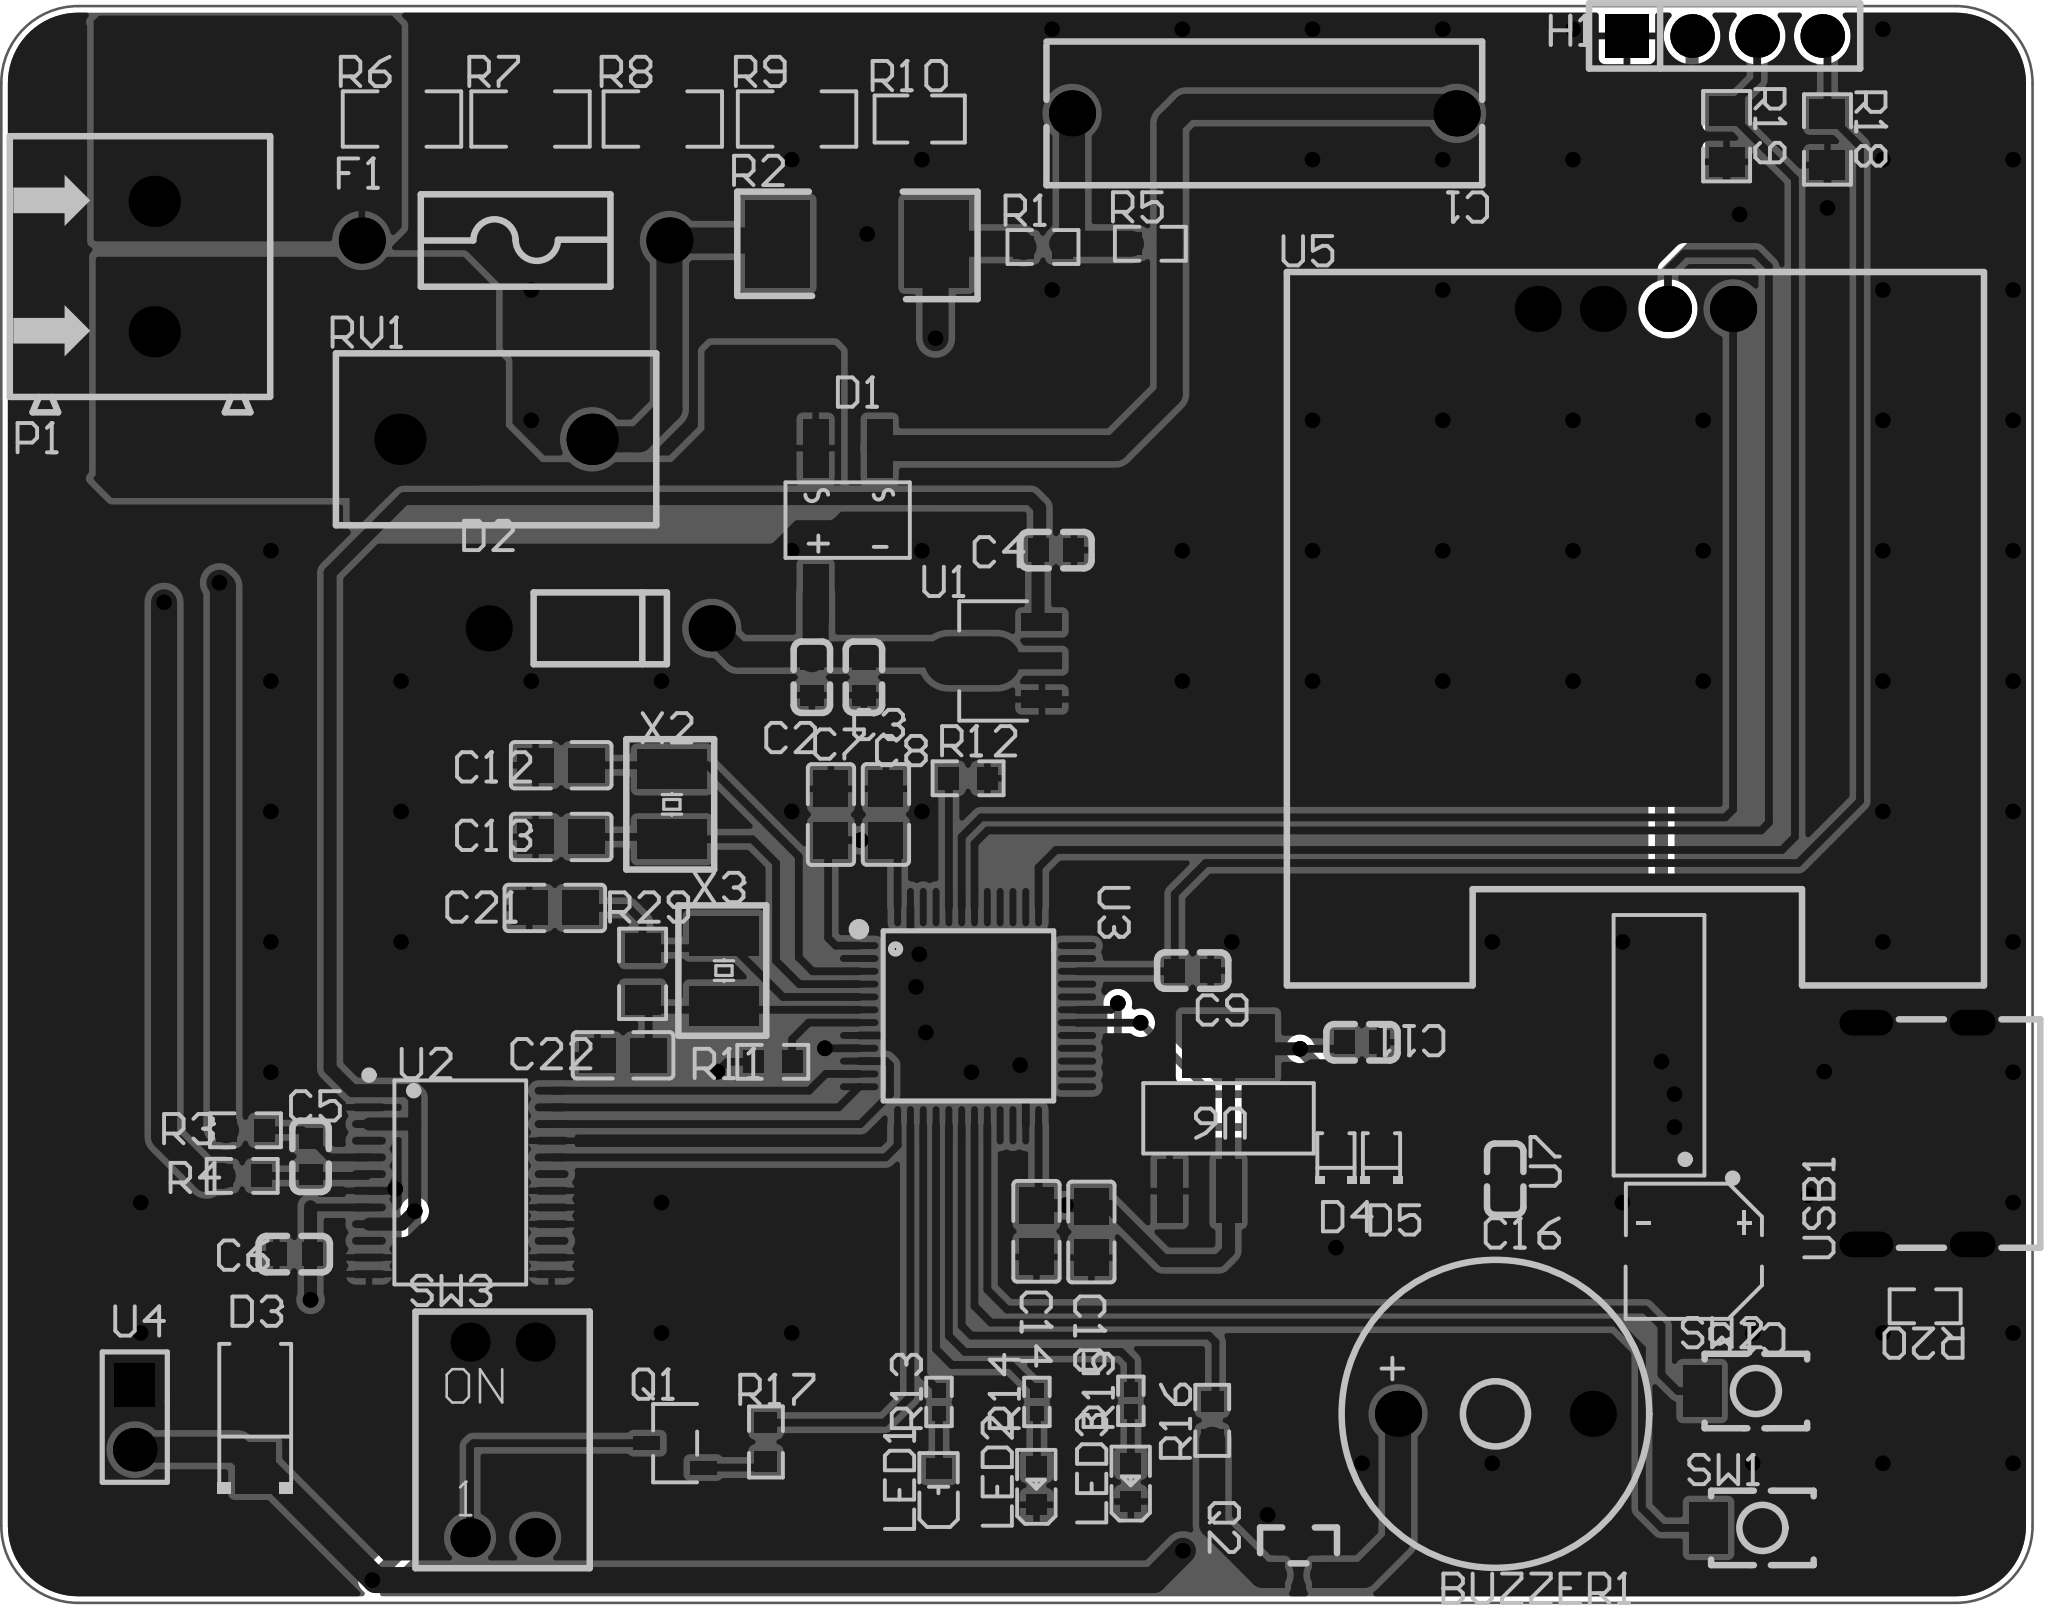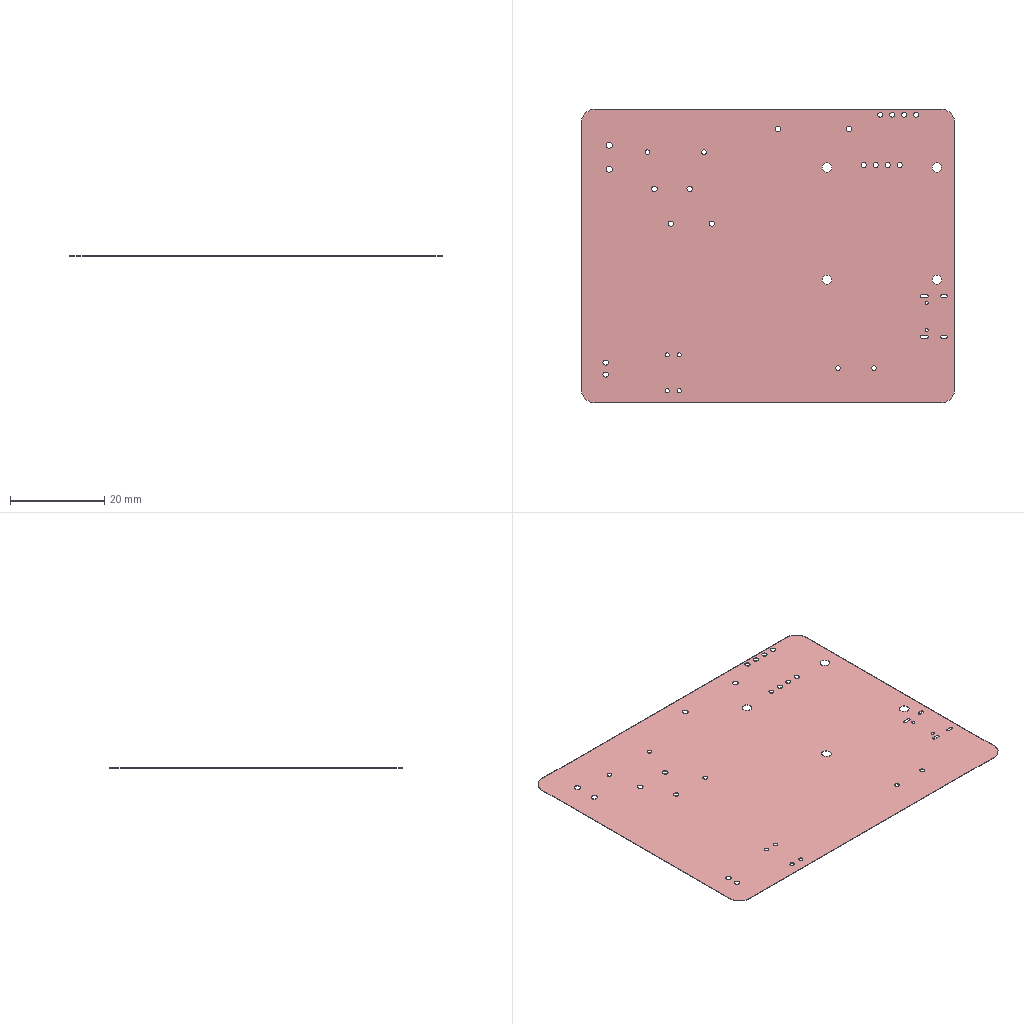Circuit board layout | Altium Designer | box 79.2 x 62.2 x 0.1 mm
Layer stack:
# Altium Designer layer stack of  (unit mm; dielectric type: 0 none, 1 core, 2 prepreg, 3 surface material)
index,name,kind,layer,copper_thickness_mm,dielectric_type,dielectric_thickness_mm,dielectric_material,dielectric_constant
0,Top Paste Mask Layer,other,,,,,,
1,Top Silkscreen Layer,other,,,,,,
2,Top Solder Mask Layer,dielectric,,,3,0.01,,3.3
3,Top Layer,copper,Top Layer,0.035,,,,
4,Bottom Layer,copper,Bottom Layer,0.035,,,,
5,Bottom Solder Mask Layer,dielectric,,,3,0.01,,3.3
6,Bottom Silkscreen Layer,other,,,,,,
7,Bottom Paste Mask Layer,other,,,,,,
# drill layer pairs: low layer,high layer
drill_pair,Top Layer,Bottom Layer
Part placement:
Designator,Comment,Layer,Footprint,Center-X(mm),Center-Y(mm),Rotation
BUZZER1,2.4kHz,TopLayer,BUZ-TH_BD12.0-P7.60-D0.6-FD,140.589,89.281,0
C1,470nF,TopLayer,CAP-TH_L17.0-W5.5-P15.00-D1.2,131.572,139.954,180
C2,100µF,TopLayer,C0603,113.919,117.983,90
C3,0.1µF,TopLayer,C0603,115.951,117.983,270
C4,10µF,TopLayer,C0603,123.444,122.936,180
C5,1nF,TopLayer,C0603,94.361,99.314,90
C6,1nF,TopLayer,C0603,93.726,95.504,0
C7,100nF,TopLayer,C0805,114.665,112.633,90
C8,100nF,TopLayer,C0805,116.809,112.637,270
C14,100nF,TopLayer,C0805,122.682,96.393,90
C10,100nF,TopLayer,C0805,124.825,96.367,270
C11,100nF,TopLayer,C0603,135.382,103.759,180
D1,MB10S,TopLayer,MBS_L4.7-W4.0-P2.50-LS7.0-TL,115.316,124.079,270
D2,1N4742,TopLayer,DO-41_BD2.4-L4.7-P8.70-D0.8-FD,105.664,119.888,0
D3,1N4007,TopLayer,SMA_L4.3-W2.5-LS5.0-RD,92.202,89.281,90
F1,2F0.05002S1B02,TopLayer,FUSE-TH_BD3.0-L7.2-P11.20-D0.6,102.362,135.001,0
LED1,NCD0603G1,TopLayer,LED0603-RD_1,118.869,86.361,90
LED2,NCD0603R1,TopLayer,LED0603-RD_RED,122.682,86.487,90
LED3,NCD0603Y1,TopLayer,LED0603-RD,126.365,86.614,90
Q1,S8050 J3Y(RANGE:200-350),TopLayer,SOT-23-3_L3.0-W1.7-P0.95-LS2.9-BR,108.585,88.138,0
R1,10Ω,TopLayer,R0603,122.936,134.747,0
R2,2mΩ,TopLayer,RES-SMD_L6.4-W3.2-1,115.697,134.874,0
R3,1K,TopLayer,R0603,91.821,100.33,0
R4,1K,TopLayer,R0603,91.694,98.552,0
R5,1MΩ,TopLayer,R0603,127.127,134.874,0
R6,1MΩ,TopLayer,R1206,97.928,139.734,0
R7,1MΩ,TopLayer,R1206,102.943,139.734,0
R8,1MΩ,TopLayer,R1206,108.104,139.734,0
R9,1MΩ,TopLayer,R1206,113.342,139.734,0
R10,10kΩ,TopLayer,R0805,118.127,139.734,0
R11,10K,TopLayer,R0603,112.395,102.997,0
R12,10K,TopLayer,R0603,120.015,114.046,0
R13,220Ω,TopLayer,R0402,118.879,89.745,90
R14,220Ω,TopLayer,R0402,122.7,89.745,90
R15,220Ω,TopLayer,R0402,126.365,89.789,90
R16,1KΩ,TopLayer,R0603,129.54,89.027,90
R17,1KΩ,TopLayer,R0603,112.128,88.184,270
RV1,190pF@1kHz,TopLayer,RES-TH_L12.5-W6.7-P7.50-D1.2,101.6,127.254,0
SW1,TS3425A2P 250gf,TopLayer,SW-SMD_L3.9-W2.9-LS5.0,151.003,84.836,0
SW2,TS3425A2P 250gf,TopLayer,SW-SMD_L3.9-W2.9-LS5.0,150.749,90.17,0
SW3,BSE02GR,TopLayer,SW-TH_4P-L9.9-W6.8-P7.62-BL,101.854,88.265,0
U1,HT7550-1,TopLayer,SOT-89_L4.5-W2.5-P1.50-LS4.2-BR,121.734,118.618,0
U2,ADE7755ARSZ,TopLayer,SSOP-24_L8.1-W5.3-P0.65-LS7.8-BL,100.203,98.298,270
U3,STM32F030C8T6TR,TopLayer,LQFP-48_L7.0-W7.0-P0.50-LS9.0-BL,120.015,104.775,270
U5,HS96L03W2C03,TopLayer,OLED-TH_L27.8-W27.2-P2.54_C9900033791,146.05,132.334,0
U6,AMS1117-3.3,TopLayer,SOT-223-4_L6.5-W3.5-P2.30-LS7.0-BR,130.175,100.796,270
P1,WJ500V-5.08-2P,TopLayer,CONN-TH_2P-P5.00_WJ500V-5.08-2P,88.265,133.985,90
U4,KF301-5.0-2P,TopLayer,HDR-M-2.54_1X2,87.503,89.154,270
C12,20pF,TopLayer,C0805,104.14,114.554,180
C13,20pF,TopLayer,C0805,104.14,111.76,0
C21,20pF,TopLayer,C0805,103.891,108.994,0
C22,20pF,TopLayer,C0805,106.553,103.251,0
R29,1M,TopLayer,R0805,107.315,106.426,90
X2,32.768MHz,TopLayer,CRYSTAL-SMD_L3.2-W2.5_3225-8MHZ,108.458,113.03,90
X3,8MHz,TopLayer,CRYSTAL-SMD_L3.2-W2.5_3225-8MHZ,110.49,106.553,90
C9,100nF,TopLayer,C0603,128.778,106.553,180
C15,10uF,TopLayer,CAP-SMD_BD5.0-L5.3-W5.3-FD,148.327,95.631,180
C16,100nF,TopLayer,C0603,140.97,98.425,90
R18,10kΩ,TopLayer,R0805,153.543,138.938,270
R19,10kΩ,TopLayer,R0805,149.606,139.065,270
R20,5.1K,TopLayer,R0603,157.353,93.472,180
U7,CH340C,TopLayer,SOP-16_L10.0-W3.9-P1.27-LS6.0-BL,146.97,103.642,90
USB1,TYPE-C16PIN,TopLayer,USB-C-SMD_TYPE-C16PIN,156.845,100.203,90
Q2,,TopLayer,S8050_SOT-23,132.906,84.154,270
H1,,TopLayer,HDR-TH_4P-P2.54-V-F,149.53,142.971,0
D4,1N5819WS,TopLayer,SOD-323_L1.8-W1.3-LS2.5-RD,134.366,99.314,90
D5,1N5819WS,TopLayer,SOD-323_L1.8-W1.3-LS2.5-RD,136.144,99.314,90
Pad and via stacks:
# Altium Designer via and pad stacks of  (unit mm). Each distinct definition once, with the count of objects using it.
# via: kind,start_layer,end_layer,hole_mm,diameter_mm,mode(0 simple;1 top-mid-bottom;2 full stack),diameter_per_layer,count,example_net
# pad: kind,layer,hole_mm,hole_type(0 round;1 square;2 slot),plating,top_size,top_shape(1 round;2 rect;3 octagon;9 rounded rect),mid_size,bottom_size,mode,footprint,size_per_layer,count,example
pad,Multi-Layer,1,0,plated,1.8x1.8,1,1.8x1.8,1.8x1.8,0,BUZ-TH_BD12.0-P7.60-D0.6-FD,,2,BUZZER1.2
pad,Multi-Layer,1.2,0,plated,1.8x1.8,1,1.8x1.8,1.8x1.8,0,CAP-TH_L17.0-W5.5-P15.00-D1.2,,2,C1.1
pad,Multi-Layer,1.1,0,plated,1.8x1.8,1,1.8x1.8,1.8x1.8,0,DO-41_BD2.4-L4.7-P8.70-D0.8-FD,,2,D2.1
pad,Multi-Layer,1,0,plated,1.8x1.8,1,1.8x1.8,1.8x1.8,0,FUSE-TH_BD3.0-L7.2-P11.20-D0.6,,2,F1.1
pad,Multi-Layer,1.2,0,plated,2x2,1,2x2,2x2,0,RES-TH_L12.5-W6.7-P7.50-D1.2,,2,RV1.1
pad,Multi-Layer,0.9144,0,plated,1.524x1.524,1,1.524x1.524,1.524x1.524,0,SW-TH_4P-L9.9-W6.8-P7.62-BL,,4,SW3.1
pad,Multi-Layer,1.05,0,plated,1.8x1.8,1,1.8x1.8,1.8x1.8,0,OLED-TH_L27.8-W27.2-P2.54_C9900033791,,4,U5.1
pad,Multi-Layer,1.3,0,plated,2x2,1,2x2,2x2,0,CONN-TH_2P-P5.00_WJ500V-5.08-2P,,2,P1.2
pad,Multi-Layer,1.1,0,plated,1.7x1.575,2,1.7x1.575,1.7x1.575,0,HDR-M-2.54_1X2,,1,U4.1
pad,Multi-Layer,1.1,0,plated,1.7x1.7,1,1.7x1.7,1.7x1.7,0,HDR-M-2.54_1X2,,1,U4.2
pad,Multi-Layer,0.6,2,plated,1x1.8,1,1x1.8,1x1.8,0,USB-C-SMD_TYPE-C16PIN,,2,USB1.4
pad,Multi-Layer,0.6,2,plated,1x2.1,1,1x2.1,1x2.1,0,USB-C-SMD_TYPE-C16PIN,,2,USB1.2
pad,Multi-Layer,1.1,0,plated,1.7x1.7,2,1.7x1.7,1.7x1.7,0,HDR-TH_4P-P2.54-V-F,,1,H1.1
pad,Multi-Layer,1.1,0,plated,1.7x1.7,1,1.7x1.7,1.7x1.7,0,HDR-TH_4P-P2.54-V-F,,3,H1.2
pad,Top Layer,0,0,plated,0.8x0.9,2,0.8x0.9,0.8x0.9,0,C0603,,16,C2.2
pad,Top Layer,0,0,plated,1.41x1.35,2,1.41x1.35,1.41x1.35,0,C0805,,16,C7.2
pad,Top Layer,0,0,plated,0.98x2.265,2,0.98x2.265,0.98x2.265,0,MBS_L4.7-W4.0-P2.50-LS7.0-TL,,4,D1.1
pad,Top Layer,0,0,plated,2x1.593,2,2x1.593,2x1.593,0,SMA_L4.3-W2.5-LS5.0-RD,,2,D3.2
pad,Top Layer,0,0,plated,1x0.8,2,1x0.8,1x0.8,0,LED0603-RD_1,,2,LED1.2
pad,Top Layer,0,0,plated,0.8x0.8,2,0.8x0.8,0.8x0.8,0,LED0603-RD_RED,,2,LED2.1
pad,Top Layer,0,0,plated,0.8x0.8,2,0.8x0.8,0.8x0.8,0,LED0603-RD,,2,LED3.2
pad,Top Layer,0,0,plated,1.038x0.532,2,1.038x0.532,1.038x0.532,0,SOT-23-3_L3.0-W1.7-P0.95-LS2.9-BR,,3,Q1.1
pad,Top Layer,0,0,plated,0.8065x0.864,2,0.8065x0.864,0.8065x0.864,0,R0603,,18,R1.2
pad,Top Layer,0,0,plated,2.5x3.4,2,2.5x3.4,2.5x3.4,0,RES-SMD_L6.4-W3.2-1,,2,R2.2
pad,Top Layer,0,0,plated,1.208x1.701,2,1.208x1.701,1.208x1.701,0,R1206,,8,R6.2
pad,Top Layer,0,0,plated,1.133x1.377,2,1.133x1.377,1.133x1.377,0,R0805,,8,R10.2
pad,Top Layer,0,0,plated,0.5657x0.54,2,0.5657x0.54,0.5657x0.54,0,R0402,,6,R13.2
pad,Top Layer,0,0,plated,1.5x2,2,1.5x2,1.5x2,0,SW-SMD_L3.9-W2.9-LS5.0,,4,SW1.1
pad,Top Layer,0,0,plated,0.95x0.95,1,0.95x0.95,0.95x0.95,0,SOT-89_L4.5-W2.5-P1.50-LS4.2-BR,,1,U1.2
pad,Top Layer,0,0,plated,1.575x0.672,2,1.575x0.672,1.575x0.672,0,SOT-89_L4.5-W2.5-P1.50-LS4.2-BR,,2,U1.3
pad,Top Layer,0,0,plated,0.308x1.324,1,0.308x1.324,0.308x1.324,0,SSOP-24_L8.1-W5.3-P0.65-LS7.8-BL,,24,U2.1
pad,Top Layer,0,0,plated,0.27x1.5,1,0.27x1.5,0.27x1.5,0,LQFP-48_L7.0-W7.0-P0.50-LS9.0-BL,,24,U3.1
pad,Top Layer,0,0,plated,1.5x0.27,1,1.5x0.27,1.5x0.27,0,LQFP-48_L7.0-W7.0-P0.50-LS9.0-BL,,24,U3.13
pad,Top Layer,0,0,plated,2.47x0.98,2,2.47x0.98,2.47x0.98,0,SOT-223-4_L6.5-W3.5-P2.30-LS7.0-BR,,3,U6.1
pad,Top Layer,0,0,plated,2.47x3.6,2,2.47x3.6,2.47x3.6,0,SOT-223-4_L6.5-W3.5-P2.30-LS7.0-BR,,1,U6.4
pad,Top Layer,0,0,plated,1.524x2.7,2,1.524x2.7,1.524x2.7,0,CRYSTAL-SMD_L3.2-W2.5_3225-8MHZ,,4,X2.1
pad,Top Layer,0,0,plated,2.8x1.1,2,2.8x1.1,2.8x1.1,0,CAP-SMD_BD5.0-L5.3-W5.3-FD,,2,C15.1
pad,Top Layer,0,0,plated,0.56x1.745,1,0.56x1.745,0.56x1.745,0,SOP-16_L10.0-W3.9-P1.27-LS6.0-BL,,16,U7.1
pad,Top Layer,0,0,plated,0.6x1.15,2,0.6x1.15,0.6x1.15,0,USB-C-SMD_TYPE-C16PIN,,4,USB1.A1B12
pad,Top Layer,0,0,plated,0.3x1.15,2,0.3x1.15,0.3x1.15,0,USB-C-SMD_TYPE-C16PIN,,8,USB1.B5
pad,Top Layer,0,0,plated,1x0.8,2,1x0.8,1x0.8,0,S8050_SOT-23,,3,Q2.2
pad,Top Layer,0,0,plated,1x0.75,2,1x0.75,1x0.75,0,SOD-323_L1.8-W1.3-LS2.5-RD,,4,D4.1
via,Top Layer,Bottom Layer,0.3048,0.6096,0,,106,TT1
Copper pours:
name,layer,net,type(0 solid;1 hatched;2 none)
Top Layer-$1N1,Top Layer,$1N1,0
Top Layer-$1N67,Top Layer,$1N67,0
Top Layer-$1N68,Top Layer,$1N68,0
Top Layer-$1N69,Top Layer,$1N69,0
Top Layer-VDDS,Top Layer,VDDS,0
Top Layer-$1N109,Top Layer,$1N109,0
Top Layer-$1N109 1,Top Layer,$1N109,0
Top Layer-GND,Top Layer,GND,0
Bottom Layer-GND,Bottom Layer,GND,0
Design rules, without the lines most boards share:
# Altium Designer design rules of  (exported by Altium Designer, unit mm)
# columns: name | kind | enabled | priority | scope1 | scope2 | descriptor | typed fields (field=value)
Plane_innerPlane | 0 | disabled | 1 | All | All | Clearance Constraint (Gap=6mil) (Disabled)(All),(All) | gap=0.1524
Plane_innerPlane_1 | 63 | disabled | 1 | All | All | Board Clearance Constraint (Gap=0mil) (Disabled)(All) |
Copper_copperRegion | 0 | disabled | 2 | All | All | Clearance Constraint (Gap=6mil) (Disabled)(All),(All) | gap=0.1524
Copper_copperRegion_1 | 63 | disabled | 2 | All | All | Board Clearance Constraint (Gap=0mil) (Disabled)(All) |
Copper_copperRegion_copperThickness1oz | 0 | disabled | 3 | All | All | Clearance Constraint (Gap=6mil) (Disabled)(All),(All) | gap=0.1524
Copper_copperRegion_copperThickness1oz_1 | 63 | disabled | 3 | All | All | Board Clearance Constraint (Gap=0mil) (Disabled)(All) |
Copper_copperRegion_Copper_copperRegion | 0 | disabled | 4 | All | All | Clearance Constraint (Gap=6mil) (Disabled)(All),(All) | gap=0.1524
Copper_copperRegion_Copper_copperRegion_1 | 63 | disabled | 4 | All | All | Board Clearance Constraint (Gap=0mil) (Disabled)(All) |
copperThickness1oz | 0 | enabled | 5 | All | All | Clearance Constraint (Gap=6mil) (All),(All) | gap=0.1524
copperThickness1oz_1 | 63 | enabled | 5 | All | All | Board Clearance Constraint (Gap=0mil) (All) |
otherClearance | 52 | enabled | 1 | All | All | Hole To Hole Clearance (Gap=11.8mil) (All),(All) | gap=0.2997
copperThickness1oz_2 | 2 | enabled | 1 | All | All | Width Constraint (Min=5mil) (Max=100mil) (Preferred=10mil) (All) |
differentialPair | 51 | enabled | 1 | All | All | Differential Pairs Uncoupled Length using the Gap Constraints (Min=5mil) (Max=6mil) (Prefered=6mil)  and Width Constraints (Min=5mil) (Max=100mil) (Prefered=100mil) (All) |
viaSize | 11 | enabled | 1 | All | All | Routing Via (MinHoleWidth=1mil) (MaxHoleWidth=393.7mil) (PreferredHoleWidth=12mil) (MinWidth=1mil) (MaxWidth=248mil) (PreferedWidth=24mil) (All) | via_min_hole=0.0254 via_max_hole=10 via_preferred_diameter=0.6096 via_preferred_hole=0.3048
copperRegion_copperThickness1oz | 20 | disabled | 1 | All | All | Polygon Connect Rule(Relief Connect )(Conductor Width=10mil) (Relief Angle=90 Angle) (Entries=4) (Air Gap Width=10mil) (Disabled)(All),(All) | connect_style(0=relief,1=direct,2=none)=0 relief_conductor_width=0.254 relief_entries=4
copperRegion_Copper_copperRegion | 20 | disabled | 2 | All | All | Polygon Connect Rule(Relief Connect )(Conductor Width=10mil) (Relief Angle=90 Angle) (Entries=4) (Air Gap Width=10mil) (Disabled)(All),(All) | connect_style(0=relief,1=direct,2=none)=0 relief_conductor_width=0.254 relief_entries=4
copperRegion | 20 | enabled | 3 | All | All | Polygon Connect Rule(Direct Connect )(Conductor Width=10mil) (Relief Angle=90 Angle) (Entries=4) (Air Gap Width=10mil) (All),(All) | connect_style(0=relief,1=direct,2=none)=1 relief_conductor_width=0.254 relief_entries=4